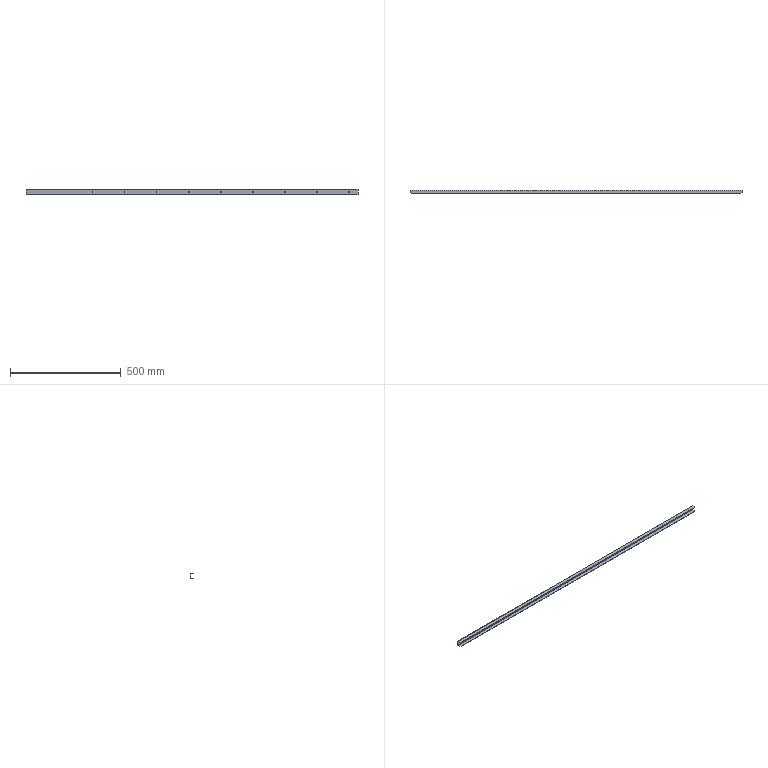Part | STEP file | b-016 | 1 solid | 44 faces | box 1500 x 16.5 x 23 mm | volume 116188 mm3 | cylinder 22 | plane 22 | commonest cylinder face diameters 3.3 x18 1.473 x2 4.473 x2